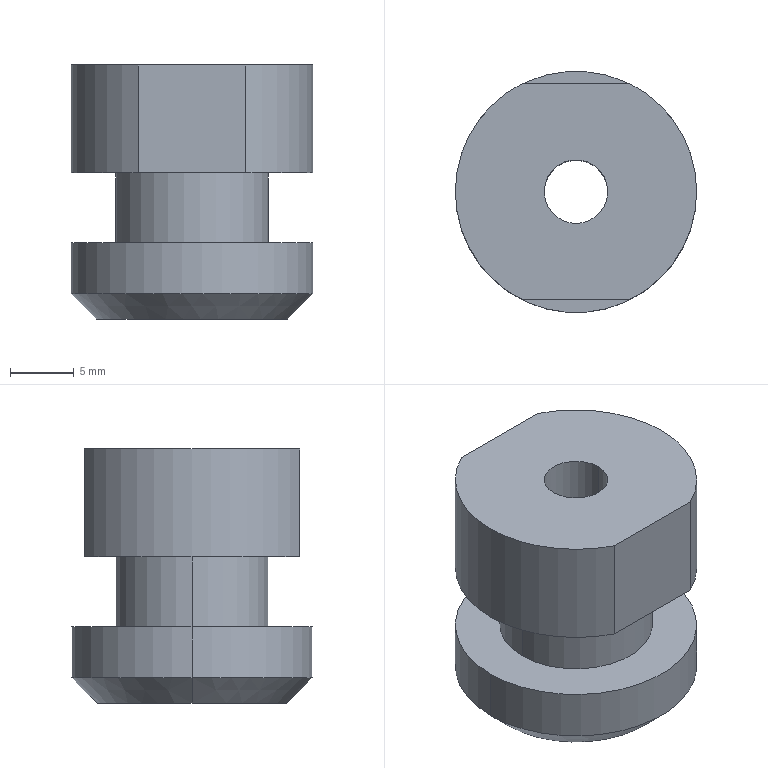Part | NX | 1 solid | 19 faces | box 19 x 19 x 20 mm | volume 4128 mm3 | cylinder 9 | plane 6 | cone 4 | commonest cylinder face diameters 19 x5 5 x2 12 x2
STEP:
#1=CARTESIAN_POINT('',(-94.033,-7.21,239.7));
#2=VERTEX_POINT('',#1);
#3=CARTESIAN_POINT('',(-94.033,-7.21,231.2));
#4=VERTEX_POINT('',#3);
#5=CARTESIAN_POINT('',(-94.033,-7.21,236.7));
#6=DIRECTION('',(0.,0.,-1.));
#7=VECTOR('',#6,1000.);
#8=LINE('',#5,#7);
#9=EDGE_CURVE('',#2,#4,#8,.T.);
#10=ORIENTED_EDGE('',*,*,#9,.F.);
#11=CARTESIAN_POINT('',(-99.29,-15.71,239.7));
#12=VERTEX_POINT('',#11);
#13=CARTESIAN_POINT('',(-103.533,-7.21,239.7));
#14=DIRECTION('',(0.,0.,1.));
#15=DIRECTION('',(1.,0.,0.));
#16=AXIS2_PLACEMENT_3D('',#13,#14,#15);
#17=CIRCLE('',#16,9.5);
#18=EDGE_CURVE('',#12,#2,#17,.T.);
#19=ORIENTED_EDGE('',*,*,#18,.F.);
#20=CARTESIAN_POINT('',(-99.29,-15.71,231.2));
#21=VERTEX_POINT('',#20);
#22=CARTESIAN_POINT('',(-99.29,-15.71,236.7));
#23=DIRECTION('',(0.,0.,-1.));
#24=VECTOR('',#23,1000.);
#25=LINE('',#22,#24);
#26=EDGE_CURVE('',#12,#21,#25,.T.);
#27=ORIENTED_EDGE('',*,*,#26,.T.);
#28=CARTESIAN_POINT('',(-103.533,-7.21,231.2));
#29=DIRECTION('',(0.,0.,1.));
#30=DIRECTION('',(1.,0.,0.));
#31=AXIS2_PLACEMENT_3D('',#28,#29,#30);
#32=CIRCLE('',#31,9.5);
#33=EDGE_CURVE('',#21,#4,#32,.T.);
#34=ORIENTED_EDGE('',*,*,#33,.T.);
#35=EDGE_LOOP('',(#10,#19,#27,#34));
#36=FACE_BOUND('',#35,.T.);
#37=CARTESIAN_POINT('',(-103.533,-7.21,236.7));
#38=DIRECTION('',(0.,0.,-1.));
#39=DIRECTION('',(1.,0.,0.));
#40=AXIS2_PLACEMENT_3D('',#37,#38,#39);
#41=CYLINDRICAL_SURFACE('',#40,9.5);
#42=ADVANCED_FACE('',(#36),#41,.T.);
#43=CARTESIAN_POINT('',(-107.775,1.29,231.2));
#44=VERTEX_POINT('',#43);
#45=CARTESIAN_POINT('',(-107.775,-15.71,231.2));
#46=VERTEX_POINT('',#45);
#47=CARTESIAN_POINT('',(-103.533,-7.21,231.2));
#48=DIRECTION('',(0.,0.,1.));
#49=DIRECTION('',(1.,0.,0.));
#50=AXIS2_PLACEMENT_3D('',#47,#48,#49);
#51=CIRCLE('',#50,9.5);
#52=EDGE_CURVE('',#44,#46,#51,.T.);
#53=ORIENTED_EDGE('',*,*,#52,.T.);
#54=CARTESIAN_POINT('',(-107.775,-15.71,239.7));
#55=VERTEX_POINT('',#54);
#56=CARTESIAN_POINT('',(-107.775,-15.71,236.7));
#57=DIRECTION('',(0.,0.,-1.));
#58=VECTOR('',#57,1000.);
#59=LINE('',#56,#58);
#60=EDGE_CURVE('',#55,#46,#59,.T.);
#61=ORIENTED_EDGE('',*,*,#60,.F.);
#62=CARTESIAN_POINT('',(-107.775,1.29,239.7));
#63=VERTEX_POINT('',#62);
#64=CARTESIAN_POINT('',(-103.533,-7.21,239.7));
#65=DIRECTION('',(0.,0.,1.));
#66=DIRECTION('',(1.,0.,0.));
#67=AXIS2_PLACEMENT_3D('',#64,#65,#66);
#68=CIRCLE('',#67,9.5);
#69=EDGE_CURVE('',#63,#55,#68,.T.);
#70=ORIENTED_EDGE('',*,*,#69,.F.);
#71=CARTESIAN_POINT('',(-107.775,1.29,236.7));
#72=DIRECTION('',(0.,0.,-1.));
#73=VECTOR('',#72,1000.);
#74=LINE('',#71,#73);
#75=EDGE_CURVE('',#63,#44,#74,.T.);
#76=ORIENTED_EDGE('',*,*,#75,.T.);
#77=EDGE_LOOP('',(#53,#61,#70,#76));
#78=FACE_BOUND('',#77,.T.);
#79=CARTESIAN_POINT('',(-103.533,-7.21,236.7));
#80=DIRECTION('',(0.,0.,-1.));
#81=DIRECTION('',(1.,0.,0.));
#82=AXIS2_PLACEMENT_3D('',#79,#80,#81);
#83=CYLINDRICAL_SURFACE('',#82,9.5);
#84=ADVANCED_FACE('',(#78),#83,.T.);
#85=ORIENTED_EDGE('',*,*,#60,.T.);
#86=CARTESIAN_POINT('',(0.,-15.71,231.2));
#87=DIRECTION('',(-1.,0.,0.));
#88=VECTOR('',#87,1000.);
#89=LINE('',#86,#88);
#90=EDGE_CURVE('',#21,#46,#89,.T.);
#91=ORIENTED_EDGE('',*,*,#90,.F.);
#92=ORIENTED_EDGE('',*,*,#26,.F.);
#93=CARTESIAN_POINT('',(0.,-15.71,239.7));
#94=DIRECTION('',(1.,0.,0.));
#95=VECTOR('',#94,1000.);
#96=LINE('',#93,#95);
#97=EDGE_CURVE('',#55,#12,#96,.T.);
#98=ORIENTED_EDGE('',*,*,#97,.F.);
#99=EDGE_LOOP('',(#85,#91,#92,#98));
#100=FACE_BOUND('',#99,.T.);
#101=CARTESIAN_POINT('',(-99.791,-15.71,236.7));
#102=DIRECTION('',(0.,1.,0.));
#103=DIRECTION('',(1.,0.,0.));
#104=AXIS2_PLACEMENT_3D('',#101,#102,#103);
#105=PLANE('',#104);
#106=ADVANCED_FACE('',(#100),#105,.F.);
#107=CARTESIAN_POINT('',(-99.29,1.29,239.7));
#108=VERTEX_POINT('',#107);
#109=CARTESIAN_POINT('',(0.,1.29,239.7));
#110=DIRECTION('',(-1.,0.,0.));
#111=VECTOR('',#110,1000.);
#112=LINE('',#109,#111);
#113=EDGE_CURVE('',#108,#63,#112,.T.);
#114=ORIENTED_EDGE('',*,*,#113,.T.);
#115=ORIENTED_EDGE('',*,*,#69,.T.);
#116=ORIENTED_EDGE('',*,*,#97,.T.);
#117=ORIENTED_EDGE('',*,*,#18,.T.);
#118=CARTESIAN_POINT('',(-103.533,-7.21,239.7));
#119=DIRECTION('',(0.,0.,1.));
#120=DIRECTION('',(1.,0.,0.));
#121=AXIS2_PLACEMENT_3D('',#118,#119,#120);
#122=CIRCLE('',#121,9.5);
#123=EDGE_CURVE('',#2,#108,#122,.T.);
#124=ORIENTED_EDGE('',*,*,#123,.T.);
#125=EDGE_LOOP('',(#114,#115,#116,#117,#124));
#126=FACE_BOUND('',#125,.T.);
#127=CARTESIAN_POINT('',(-106.033,-7.21,239.7));
#128=VERTEX_POINT('',#127);
#129=CARTESIAN_POINT('',(-101.033,-7.21,239.7));
#130=VERTEX_POINT('',#129);
#131=CARTESIAN_POINT('',(-103.533,-7.21,239.7));
#132=DIRECTION('',(0.,0.,-1.));
#133=DIRECTION('',(-1.,0.,0.));
#134=AXIS2_PLACEMENT_3D('',#131,#132,#133);
#135=CIRCLE('',#134,2.5);
#136=EDGE_CURVE('',#128,#130,#135,.T.);
#137=ORIENTED_EDGE('',*,*,#136,.T.);
#138=CARTESIAN_POINT('',(-103.533,-7.21,239.7));
#139=DIRECTION('',(0.,0.,-1.));
#140=DIRECTION('',(-1.,0.,0.));
#141=AXIS2_PLACEMENT_3D('',#138,#139,#140);
#142=CIRCLE('',#141,2.5);
#143=EDGE_CURVE('',#130,#128,#142,.T.);
#144=ORIENTED_EDGE('',*,*,#143,.T.);
#145=EDGE_LOOP('',(#137,#144));
#146=FACE_BOUND('',#145,.T.);
#147=CARTESIAN_POINT('',(-104.112,-7.022,239.7));
#148=DIRECTION('',(0.,0.,1.));
#149=DIRECTION('',(1.,0.,0.));
#150=AXIS2_PLACEMENT_3D('',#147,#148,#149);
#151=PLANE('',#150);
#152=ADVANCED_FACE('',(#126,#146),#151,.T.);
#153=CARTESIAN_POINT('',(-100.083,-7.21,219.7));
#154=VERTEX_POINT('',#153);
#155=CARTESIAN_POINT('',(-106.983,-7.21,219.7));
#156=VERTEX_POINT('',#155);
#157=CARTESIAN_POINT('',(-103.533,-7.21,219.7));
#158=DIRECTION('',(0.,0.,-1.));
#159=DIRECTION('',(-1.,0.,0.));
#160=AXIS2_PLACEMENT_3D('',#157,#158,#159);
#161=CIRCLE('',#160,3.45);
#162=EDGE_CURVE('',#154,#156,#161,.T.);
#163=ORIENTED_EDGE('',*,*,#162,.T.);
#164=CARTESIAN_POINT('',(-106.033,-7.21,220.248));
#165=VERTEX_POINT('',#164);
#166=CARTESIAN_POINT('',(-106.033,-7.21,220.248));
#167=DIRECTION('',(-0.866,0.,-0.5));
#168=VECTOR('',#167,1000.);
#169=LINE('',#166,#168);
#170=EDGE_CURVE('',#156,#165,#169,.F.);
#171=ORIENTED_EDGE('',*,*,#170,.T.);
#172=CARTESIAN_POINT('',(-101.033,-7.21,220.248));
#173=VERTEX_POINT('',#172);
#174=CARTESIAN_POINT('',(-103.533,-7.21,220.248));
#175=DIRECTION('',(0.,0.,-1.));
#176=DIRECTION('',(-1.,0.,0.));
#177=AXIS2_PLACEMENT_3D('',#174,#175,#176);
#178=CIRCLE('',#177,2.5);
#179=EDGE_CURVE('',#173,#165,#178,.T.);
#180=ORIENTED_EDGE('',*,*,#179,.F.);
#181=CARTESIAN_POINT('',(-101.033,-7.21,220.248));
#182=DIRECTION('',(0.866,0.,-0.5));
#183=VECTOR('',#182,1000.);
#184=LINE('',#181,#183);
#185=EDGE_CURVE('',#154,#173,#184,.F.);
#186=ORIENTED_EDGE('',*,*,#185,.F.);
#187=EDGE_LOOP('',(#163,#171,#180,#186));
#188=FACE_BOUND('',#187,.T.);
#189=CARTESIAN_POINT('',(-103.533,-7.21,220.248));
#190=DIRECTION('',(0.,0.,-1.));
#191=DIRECTION('',(-1.,0.,0.));
#192=AXIS2_PLACEMENT_3D('',#189,#190,#191);
#193=CONICAL_SURFACE('',#192,2.5,1.047);
#194=ADVANCED_FACE('',(#188),#193,.F.);
#195=CARTESIAN_POINT('',(-94.033,-7.21,225.7));
#196=VERTEX_POINT('',#195);
#197=CARTESIAN_POINT('',(-113.033,-7.21,225.7));
#198=VERTEX_POINT('',#197);
#199=CARTESIAN_POINT('',(-103.533,-7.21,225.7));
#200=DIRECTION('',(0.,0.,1.));
#201=DIRECTION('',(1.,0.,0.));
#202=AXIS2_PLACEMENT_3D('',#199,#200,#201);
#203=CIRCLE('',#202,9.5);
#204=EDGE_CURVE('',#196,#198,#203,.T.);
#205=ORIENTED_EDGE('',*,*,#204,.T.);
#206=CARTESIAN_POINT('',(-103.533,-7.21,225.7));
#207=DIRECTION('',(0.,0.,1.));
#208=DIRECTION('',(1.,0.,0.));
#209=AXIS2_PLACEMENT_3D('',#206,#207,#208);
#210=CIRCLE('',#209,9.5);
#211=EDGE_CURVE('',#198,#196,#210,.T.);
#212=ORIENTED_EDGE('',*,*,#211,.T.);
#213=EDGE_LOOP('',(#205,#212));
#214=FACE_BOUND('',#213,.T.);
#215=CARTESIAN_POINT('',(-97.533,-7.21,225.7));
#216=VERTEX_POINT('',#215);
#217=CARTESIAN_POINT('',(-109.533,-7.21,225.7));
#218=VERTEX_POINT('',#217);
#219=CARTESIAN_POINT('',(-103.533,-7.21,225.7));
#220=DIRECTION('',(0.,0.,1.));
#221=DIRECTION('',(1.,0.,0.));
#222=AXIS2_PLACEMENT_3D('',#219,#220,#221);
#223=CIRCLE('',#222,6.);
#224=EDGE_CURVE('',#216,#218,#223,.T.);
#225=ORIENTED_EDGE('',*,*,#224,.F.);
#226=CARTESIAN_POINT('',(-103.533,-7.21,225.7));
#227=DIRECTION('',(0.,0.,1.));
#228=DIRECTION('',(1.,0.,0.));
#229=AXIS2_PLACEMENT_3D('',#226,#227,#228);
#230=CIRCLE('',#229,6.);
#231=EDGE_CURVE('',#218,#216,#230,.T.);
#232=ORIENTED_EDGE('',*,*,#231,.F.);
#233=EDGE_LOOP('',(#225,#232));
#234=FACE_BOUND('',#233,.T.);
#235=CARTESIAN_POINT('',(-103.03,-7.592,225.7));
#236=DIRECTION('',(0.,0.,1.));
#237=DIRECTION('',(1.,0.,0.));
#238=AXIS2_PLACEMENT_3D('',#235,#236,#237);
#239=PLANE('',#238);
#240=ADVANCED_FACE('',(#214,#234),#239,.T.);
#241=ORIENTED_EDGE('',*,*,#224,.T.);
#242=CARTESIAN_POINT('',(-109.533,-7.21,231.2));
#243=VERTEX_POINT('',#242);
#244=CARTESIAN_POINT('',(-109.533,-7.21,230.7));
#245=DIRECTION('',(0.,0.,-1.));
#246=VECTOR('',#245,1000.);
#247=LINE('',#244,#246);
#248=EDGE_CURVE('',#243,#218,#247,.T.);
#249=ORIENTED_EDGE('',*,*,#248,.F.);
#250=CARTESIAN_POINT('',(-97.533,-7.21,231.2));
#251=VERTEX_POINT('',#250);
#252=CARTESIAN_POINT('',(-103.533,-7.21,231.2));
#253=DIRECTION('',(0.,0.,1.));
#254=DIRECTION('',(1.,0.,0.));
#255=AXIS2_PLACEMENT_3D('',#252,#253,#254);
#256=CIRCLE('',#255,6.);
#257=EDGE_CURVE('',#251,#243,#256,.T.);
#258=ORIENTED_EDGE('',*,*,#257,.F.);
#259=CARTESIAN_POINT('',(-97.533,-7.21,230.7));
#260=DIRECTION('',(0.,0.,-1.));
#261=VECTOR('',#260,1000.);
#262=LINE('',#259,#261);
#263=EDGE_CURVE('',#251,#216,#262,.T.);
#264=ORIENTED_EDGE('',*,*,#263,.T.);
#265=EDGE_LOOP('',(#241,#249,#258,#264));
#266=FACE_BOUND('',#265,.T.);
#267=CARTESIAN_POINT('',(-103.533,-7.21,230.7));
#268=DIRECTION('',(0.,0.,-1.));
#269=DIRECTION('',(1.,0.,0.));
#270=AXIS2_PLACEMENT_3D('',#267,#268,#269);
#271=CYLINDRICAL_SURFACE('',#270,6.);
#272=ADVANCED_FACE('',(#266),#271,.T.);
#273=CARTESIAN_POINT('',(-111.033,-7.21,219.7));
#274=VERTEX_POINT('',#273);
#275=CARTESIAN_POINT('',(-96.033,-7.21,219.7));
#276=VERTEX_POINT('',#275);
#277=CARTESIAN_POINT('',(-103.533,-7.21,219.7));
#278=DIRECTION('',(0.,0.,1.));
#279=DIRECTION('',(1.,0.,0.));
#280=AXIS2_PLACEMENT_3D('',#277,#278,#279);
#281=CIRCLE('',#280,7.5);
#282=EDGE_CURVE('',#274,#276,#281,.T.);
#283=ORIENTED_EDGE('',*,*,#282,.F.);
#284=CARTESIAN_POINT('',(-103.533,-7.21,219.7));
#285=DIRECTION('',(0.,0.,1.));
#286=DIRECTION('',(1.,0.,0.));
#287=AXIS2_PLACEMENT_3D('',#284,#285,#286);
#288=CIRCLE('',#287,7.5);
#289=EDGE_CURVE('',#276,#274,#288,.T.);
#290=ORIENTED_EDGE('',*,*,#289,.F.);
#291=EDGE_LOOP('',(#283,#290));
#292=FACE_BOUND('',#291,.T.);
#293=ORIENTED_EDGE('',*,*,#162,.F.);
#294=CARTESIAN_POINT('',(-103.533,-7.21,219.7));
#295=DIRECTION('',(0.,0.,-1.));
#296=DIRECTION('',(-1.,0.,0.));
#297=AXIS2_PLACEMENT_3D('',#294,#295,#296);
#298=CIRCLE('',#297,3.45);
#299=EDGE_CURVE('',#156,#154,#298,.T.);
#300=ORIENTED_EDGE('',*,*,#299,.F.);
#301=EDGE_LOOP('',(#293,#300));
#302=FACE_BOUND('',#301,.T.);
#303=CARTESIAN_POINT('',(-103.03,-7.592,219.7));
#304=DIRECTION('',(0.,0.,1.));
#305=DIRECTION('',(1.,0.,0.));
#306=AXIS2_PLACEMENT_3D('',#303,#304,#305);
#307=PLANE('',#306);
#308=ADVANCED_FACE('',(#292,#302),#307,.F.);
#309=ORIENTED_EDGE('',*,*,#204,.F.);
#310=CARTESIAN_POINT('',(-94.033,-7.21,221.7));
#311=VERTEX_POINT('',#310);
#312=CARTESIAN_POINT('',(-94.033,-7.21,225.7));
#313=DIRECTION('',(0.,0.,-1.));
#314=VECTOR('',#313,1000.);
#315=LINE('',#312,#314);
#316=EDGE_CURVE('',#196,#311,#315,.T.);
#317=ORIENTED_EDGE('',*,*,#316,.T.);
#318=CARTESIAN_POINT('',(-113.033,-7.21,221.7));
#319=VERTEX_POINT('',#318);
#320=CARTESIAN_POINT('',(-103.533,-7.21,221.7));
#321=DIRECTION('',(0.,0.,1.));
#322=DIRECTION('',(1.,0.,0.));
#323=AXIS2_PLACEMENT_3D('',#320,#321,#322);
#324=CIRCLE('',#323,9.5);
#325=EDGE_CURVE('',#311,#319,#324,.T.);
#326=ORIENTED_EDGE('',*,*,#325,.T.);
#327=CARTESIAN_POINT('',(-113.033,-7.21,225.7));
#328=DIRECTION('',(0.,0.,-1.));
#329=VECTOR('',#328,1000.);
#330=LINE('',#327,#329);
#331=EDGE_CURVE('',#198,#319,#330,.T.);
#332=ORIENTED_EDGE('',*,*,#331,.F.);
#333=EDGE_LOOP('',(#309,#317,#326,#332));
#334=FACE_BOUND('',#333,.T.);
#335=CARTESIAN_POINT('',(-103.533,-7.21,225.7));
#336=DIRECTION('',(0.,0.,-1.));
#337=DIRECTION('',(1.,0.,0.));
#338=AXIS2_PLACEMENT_3D('',#335,#336,#337);
#339=CYLINDRICAL_SURFACE('',#338,9.5);
#340=ADVANCED_FACE('',(#334),#339,.T.);
#341=ORIENTED_EDGE('',*,*,#90,.T.);
#342=ORIENTED_EDGE('',*,*,#52,.F.);
#343=CARTESIAN_POINT('',(-99.29,1.29,231.2));
#344=VERTEX_POINT('',#343);
#345=CARTESIAN_POINT('',(0.,1.29,231.2));
#346=DIRECTION('',(1.,0.,0.));
#347=VECTOR('',#346,1000.);
#348=LINE('',#345,#347);
#349=EDGE_CURVE('',#44,#344,#348,.T.);
#350=ORIENTED_EDGE('',*,*,#349,.T.);
#351=CARTESIAN_POINT('',(-103.533,-7.21,231.2));
#352=DIRECTION('',(0.,0.,1.));
#353=DIRECTION('',(1.,0.,0.));
#354=AXIS2_PLACEMENT_3D('',#351,#352,#353);
#355=CIRCLE('',#354,9.5);
#356=EDGE_CURVE('',#4,#344,#355,.T.);
#357=ORIENTED_EDGE('',*,*,#356,.F.);
#358=ORIENTED_EDGE('',*,*,#33,.F.);
#359=EDGE_LOOP('',(#341,#342,#350,#357,#358));
#360=FACE_BOUND('',#359,.T.);
#361=ORIENTED_EDGE('',*,*,#257,.T.);
#362=CARTESIAN_POINT('',(-103.533,-7.21,231.2));
#363=DIRECTION('',(0.,0.,1.));
#364=DIRECTION('',(1.,0.,0.));
#365=AXIS2_PLACEMENT_3D('',#362,#363,#364);
#366=CIRCLE('',#365,6.);
#367=EDGE_CURVE('',#243,#251,#366,.T.);
#368=ORIENTED_EDGE('',*,*,#367,.T.);
#369=EDGE_LOOP('',(#361,#368));
#370=FACE_BOUND('',#369,.T.);
#371=CARTESIAN_POINT('',(-104.112,-7.022,231.2));
#372=DIRECTION('',(0.,0.,1.));
#373=DIRECTION('',(1.,0.,0.));
#374=AXIS2_PLACEMENT_3D('',#371,#372,#373);
#375=PLANE('',#374);
#376=ADVANCED_FACE('',(#360,#370),#375,.F.);
#377=CARTESIAN_POINT('',(-103.533,-7.21,221.7));
#378=DIRECTION('',(0.,0.,1.));
#379=DIRECTION('',(1.,0.,0.));
#380=AXIS2_PLACEMENT_3D('',#377,#378,#379);
#381=CIRCLE('',#380,9.5);
#382=EDGE_CURVE('',#319,#311,#381,.T.);
#383=ORIENTED_EDGE('',*,*,#382,.F.);
#384=CARTESIAN_POINT('',(-111.033,-7.21,219.7));
#385=DIRECTION('',(-0.7071,0.,0.7071));
#386=VECTOR('',#385,1000.);
#387=LINE('',#384,#386);
#388=EDGE_CURVE('',#274,#319,#387,.T.);
#389=ORIENTED_EDGE('',*,*,#388,.F.);
#390=ORIENTED_EDGE('',*,*,#282,.T.);
#391=CARTESIAN_POINT('',(-96.033,-7.21,219.7));
#392=DIRECTION('',(0.7071,0.,0.7071));
#393=VECTOR('',#392,1000.);
#394=LINE('',#391,#393);
#395=EDGE_CURVE('',#276,#311,#394,.T.);
#396=ORIENTED_EDGE('',*,*,#395,.T.);
#397=EDGE_LOOP('',(#383,#389,#390,#396));
#398=FACE_BOUND('',#397,.T.);
#399=CARTESIAN_POINT('',(-103.533,-7.21,219.7));
#400=DIRECTION('',(0.,0.,1.));
#401=DIRECTION('',(1.,0.,0.));
#402=AXIS2_PLACEMENT_3D('',#399,#400,#401);
#403=CONICAL_SURFACE('',#402,7.5,0.7854);
#404=ADVANCED_FACE('',(#398),#403,.T.);
#405=CARTESIAN_POINT('',(-99.29,1.29,236.7));
#406=DIRECTION('',(0.,0.,-1.));
#407=VECTOR('',#406,1000.);
#408=LINE('',#405,#407);
#409=EDGE_CURVE('',#108,#344,#408,.T.);
#410=ORIENTED_EDGE('',*,*,#409,.T.);
#411=ORIENTED_EDGE('',*,*,#349,.F.);
#412=ORIENTED_EDGE('',*,*,#75,.F.);
#413=ORIENTED_EDGE('',*,*,#113,.F.);
#414=EDGE_LOOP('',(#410,#411,#412,#413));
#415=FACE_BOUND('',#414,.T.);
#416=CARTESIAN_POINT('',(-107.274,1.29,236.7));
#417=DIRECTION('',(0.,-1.,0.));
#418=DIRECTION('',(0.,0.,-1.));
#419=AXIS2_PLACEMENT_3D('',#416,#417,#418);
#420=PLANE('',#419);
#421=ADVANCED_FACE('',(#415),#420,.F.);
#422=CARTESIAN_POINT('',(-103.533,-7.21,220.248));
#423=DIRECTION('',(0.,0.,-1.));
#424=DIRECTION('',(-1.,0.,0.));
#425=AXIS2_PLACEMENT_3D('',#422,#423,#424);
#426=CIRCLE('',#425,2.5);
#427=EDGE_CURVE('',#165,#173,#426,.T.);
#428=ORIENTED_EDGE('',*,*,#427,.T.);
#429=CARTESIAN_POINT('',(-101.033,-7.21,219.7));
#430=DIRECTION('',(0.,0.,-1.));
#431=VECTOR('',#430,1000.);
#432=LINE('',#429,#431);
#433=EDGE_CURVE('',#173,#130,#432,.F.);
#434=ORIENTED_EDGE('',*,*,#433,.T.);
#435=ORIENTED_EDGE('',*,*,#136,.F.);
#436=CARTESIAN_POINT('',(-106.033,-7.21,219.7));
#437=DIRECTION('',(0.,0.,-1.));
#438=VECTOR('',#437,1000.);
#439=LINE('',#436,#438);
#440=EDGE_CURVE('',#165,#128,#439,.F.);
#441=ORIENTED_EDGE('',*,*,#440,.F.);
#442=EDGE_LOOP('',(#428,#434,#435,#441));
#443=FACE_BOUND('',#442,.T.);
#444=CARTESIAN_POINT('',(-103.533,-7.21,219.7));
#445=DIRECTION('',(0.,0.,-1.));
#446=DIRECTION('',(-1.,0.,0.));
#447=AXIS2_PLACEMENT_3D('',#444,#445,#446);
#448=CYLINDRICAL_SURFACE('',#447,2.5);
#449=ADVANCED_FACE('',(#443),#448,.F.);
#450=ORIENTED_EDGE('',*,*,#440,.T.);
#451=ORIENTED_EDGE('',*,*,#143,.F.);
#452=ORIENTED_EDGE('',*,*,#433,.F.);
#453=ORIENTED_EDGE('',*,*,#179,.T.);
#454=EDGE_LOOP('',(#450,#451,#452,#453));
#455=FACE_BOUND('',#454,.T.);
#456=CARTESIAN_POINT('',(-103.533,-7.21,219.7));
#457=DIRECTION('',(0.,0.,-1.));
#458=DIRECTION('',(-1.,0.,0.));
#459=AXIS2_PLACEMENT_3D('',#456,#457,#458);
#460=CYLINDRICAL_SURFACE('',#459,2.5);
#461=ADVANCED_FACE('',(#455),#460,.F.);
#462=ORIENTED_EDGE('',*,*,#395,.F.);
#463=ORIENTED_EDGE('',*,*,#289,.T.);
#464=ORIENTED_EDGE('',*,*,#388,.T.);
#465=ORIENTED_EDGE('',*,*,#325,.F.);
#466=EDGE_LOOP('',(#462,#463,#464,#465));
#467=FACE_BOUND('',#466,.T.);
#468=CARTESIAN_POINT('',(-103.533,-7.21,219.7));
#469=DIRECTION('',(0.,0.,1.));
#470=DIRECTION('',(1.,0.,0.));
#471=AXIS2_PLACEMENT_3D('',#468,#469,#470);
#472=CONICAL_SURFACE('',#471,7.5,0.7854);
#473=ADVANCED_FACE('',(#467),#472,.T.);
#474=ORIENTED_EDGE('',*,*,#263,.F.);
#475=ORIENTED_EDGE('',*,*,#367,.F.);
#476=ORIENTED_EDGE('',*,*,#248,.T.);
#477=ORIENTED_EDGE('',*,*,#231,.T.);
#478=EDGE_LOOP('',(#474,#475,#476,#477));
#479=FACE_BOUND('',#478,.T.);
#480=CARTESIAN_POINT('',(-103.533,-7.21,230.7));
#481=DIRECTION('',(0.,0.,-1.));
#482=DIRECTION('',(1.,0.,0.));
#483=AXIS2_PLACEMENT_3D('',#480,#481,#482);
#484=CYLINDRICAL_SURFACE('',#483,6.);
#485=ADVANCED_FACE('',(#479),#484,.T.);
#486=ORIENTED_EDGE('',*,*,#427,.F.);
#487=ORIENTED_EDGE('',*,*,#170,.F.);
#488=ORIENTED_EDGE('',*,*,#299,.T.);
#489=ORIENTED_EDGE('',*,*,#185,.T.);
#490=EDGE_LOOP('',(#486,#487,#488,#489));
#491=FACE_BOUND('',#490,.T.);
#492=CARTESIAN_POINT('',(-103.533,-7.21,220.248));
#493=DIRECTION('',(0.,0.,-1.));
#494=DIRECTION('',(-1.,0.,0.));
#495=AXIS2_PLACEMENT_3D('',#492,#493,#494);
#496=CONICAL_SURFACE('',#495,2.5,1.047);
#497=ADVANCED_FACE('',(#491),#496,.F.);
#498=ORIENTED_EDGE('',*,*,#382,.T.);
#499=ORIENTED_EDGE('',*,*,#316,.F.);
#500=ORIENTED_EDGE('',*,*,#211,.F.);
#501=ORIENTED_EDGE('',*,*,#331,.T.);
#502=EDGE_LOOP('',(#498,#499,#500,#501));
#503=FACE_BOUND('',#502,.T.);
#504=CARTESIAN_POINT('',(-103.533,-7.21,225.7));
#505=DIRECTION('',(0.,0.,-1.));
#506=DIRECTION('',(1.,0.,0.));
#507=AXIS2_PLACEMENT_3D('',#504,#505,#506);
#508=CYLINDRICAL_SURFACE('',#507,9.5);
#509=ADVANCED_FACE('',(#503),#508,.T.);
#510=ORIENTED_EDGE('',*,*,#123,.F.);
#511=ORIENTED_EDGE('',*,*,#9,.T.);
#512=ORIENTED_EDGE('',*,*,#356,.T.);
#513=ORIENTED_EDGE('',*,*,#409,.F.);
#514=EDGE_LOOP('',(#510,#511,#512,#513));
#515=FACE_BOUND('',#514,.T.);
#516=CARTESIAN_POINT('',(-103.533,-7.21,236.7));
#517=DIRECTION('',(0.,0.,-1.));
#518=DIRECTION('',(1.,0.,0.));
#519=AXIS2_PLACEMENT_3D('',#516,#517,#518);
#520=CYLINDRICAL_SURFACE('',#519,9.5);
#521=ADVANCED_FACE('',(#515),#520,.T.);
#522=CLOSED_SHELL('',(#42,#84,#106,#152,#194,#240,#272,#308,#340,#376,#404,#421,#449,#461,#473,#485,#497,#509,#521));
#523=MANIFOLD_SOLID_BREP('',#522);
#524=(LENGTH_UNIT()NAMED_UNIT(*)SI_UNIT(.MILLI.,.METRE.));
#525=UNCERTAINTY_MEASURE_WITH_UNIT(LENGTH_MEASURE(0.00001),#524,'','');
#526=(NAMED_UNIT(*)PLANE_ANGLE_UNIT()SI_UNIT($,.RADIAN.));
#527=(NAMED_UNIT(*)SI_UNIT($,.STERADIAN.)SOLID_ANGLE_UNIT());
#528=(GEOMETRIC_REPRESENTATION_CONTEXT(3)GLOBAL_UNCERTAINTY_ASSIGNED_CONTEXT((#525))GLOBAL_UNIT_ASSIGNED_CONTEXT((#524,#526,#527))REPRESENTATION_CONTEXT('',''));
#529=ADVANCED_BREP_SHAPE_REPRESENTATION('',(#523),#528);